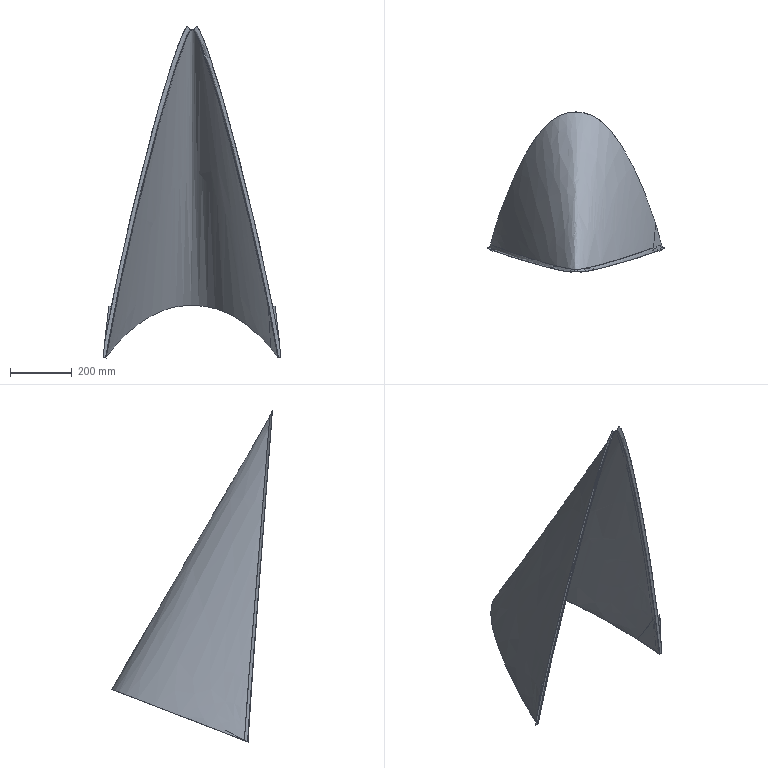Part | SolidWorks | features BaseBody 3 | 3 solids | 31 faces | box 575.61 x 521.13 x 1077 mm | volume 2626040 mm3 | spline 24 | plane 7